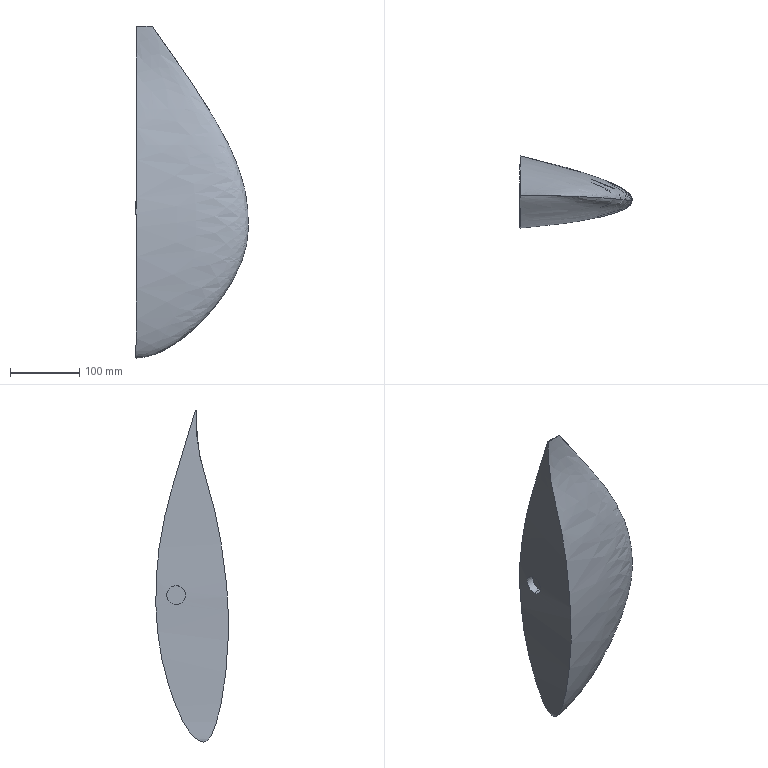Part | SolidWorks | features BaseBody 1 | 1 solid | 7 faces | box 163.209 x 104.812 x 479.995 mm | volume 2901652 mm3 | spline 3 | cylinder 2 | plane 2 | commonest cylinder face diameters 27.359 x2